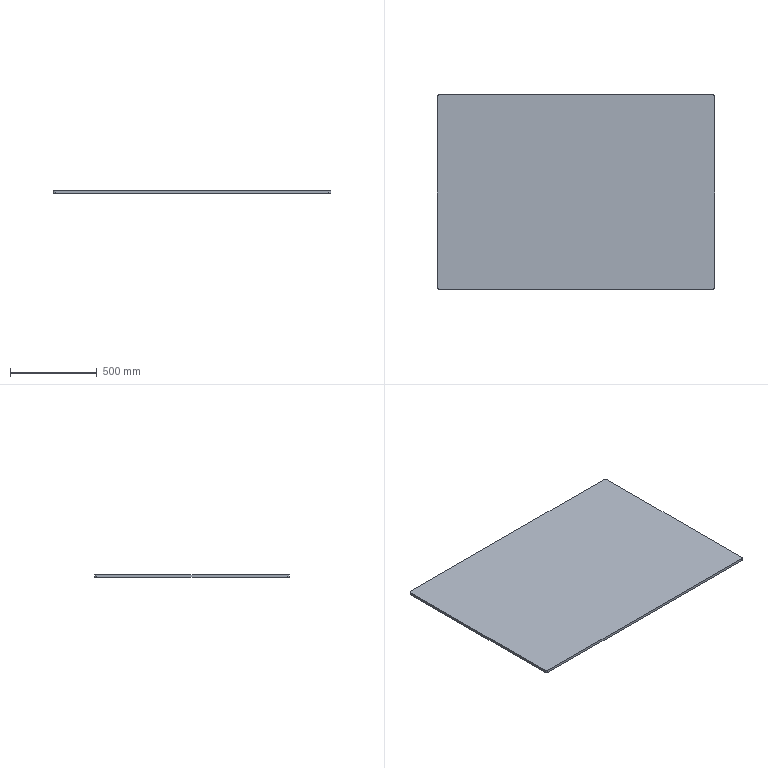Part | STEP file | Part 2 | 1 solid | 10 faces | box 1600 x 1120 x 15 mm | volume 26878712 mm3 | plane 6 | cylinder 4 | commonest cylinder face diameters 20 x4
STEP:
#1=CARTESIAN_POINT('',(800.,-550.,15.));
#2=VERTEX_POINT('',#1);
#3=CARTESIAN_POINT('',(800.,550.,15.));
#4=VERTEX_POINT('',#3);
#5=CARTESIAN_POINT('',(800.,560.,15.));
#6=DIRECTION('',(0.,1.,0.));
#7=VECTOR('',#6,1000.);
#8=LINE('',#5,#7);
#9=EDGE_CURVE('',#2,#4,#8,.T.);
#10=ORIENTED_EDGE('',*,*,#9,.F.);
#11=CARTESIAN_POINT('',(800.,-550.,0.));
#12=VERTEX_POINT('',#11);
#13=CARTESIAN_POINT('',(800.,-550.,15.));
#14=DIRECTION('',(0.,0.,-1.));
#15=VECTOR('',#14,1000.);
#16=LINE('',#13,#15);
#17=EDGE_CURVE('',#2,#12,#16,.T.);
#18=ORIENTED_EDGE('',*,*,#17,.T.);
#19=CARTESIAN_POINT('',(800.,550.,0.));
#20=VERTEX_POINT('',#19);
#21=CARTESIAN_POINT('',(800.,560.,0.));
#22=DIRECTION('',(0.,1.,0.));
#23=VECTOR('',#22,1000.);
#24=LINE('',#21,#23);
#25=EDGE_CURVE('',#12,#20,#24,.T.);
#26=ORIENTED_EDGE('',*,*,#25,.T.);
#27=CARTESIAN_POINT('',(800.,550.,15.));
#28=DIRECTION('',(0.,0.,1.));
#29=VECTOR('',#28,1000.);
#30=LINE('',#27,#29);
#31=EDGE_CURVE('',#20,#4,#30,.T.);
#32=ORIENTED_EDGE('',*,*,#31,.T.);
#33=EDGE_LOOP('',(#10,#18,#26,#32));
#34=FACE_OUTER_BOUND('',#33,.T.);
#35=CARTESIAN_POINT('',(800.,560.,15.));
#36=DIRECTION('',(-1.,0.,0.));
#37=DIRECTION('',(0.,-1.,0.));
#38=AXIS2_PLACEMENT_3D('',#35,#36,#37);
#39=PLANE('',#38);
#40=ADVANCED_FACE('',(#34),#39,.F.);
#41=CARTESIAN_POINT('',(790.,560.,15.));
#42=VERTEX_POINT('',#41);
#43=CARTESIAN_POINT('',(-790.,560.,15.));
#44=VERTEX_POINT('',#43);
#45=CARTESIAN_POINT('',(-800.,560.,15.));
#46=DIRECTION('',(-1.,0.,0.));
#47=VECTOR('',#46,1000.);
#48=LINE('',#45,#47);
#49=EDGE_CURVE('',#42,#44,#48,.T.);
#50=ORIENTED_EDGE('',*,*,#49,.F.);
#51=CARTESIAN_POINT('',(790.,560.,0.));
#52=VERTEX_POINT('',#51);
#53=CARTESIAN_POINT('',(790.,560.,15.));
#54=DIRECTION('',(0.,0.,-1.));
#55=VECTOR('',#54,1000.);
#56=LINE('',#53,#55);
#57=EDGE_CURVE('',#42,#52,#56,.T.);
#58=ORIENTED_EDGE('',*,*,#57,.T.);
#59=CARTESIAN_POINT('',(-790.,560.,0.));
#60=VERTEX_POINT('',#59);
#61=CARTESIAN_POINT('',(-800.,560.,0.));
#62=DIRECTION('',(-1.,0.,0.));
#63=VECTOR('',#62,1000.);
#64=LINE('',#61,#63);
#65=EDGE_CURVE('',#52,#60,#64,.T.);
#66=ORIENTED_EDGE('',*,*,#65,.T.);
#67=CARTESIAN_POINT('',(-790.,560.,15.));
#68=DIRECTION('',(0.,0.,1.));
#69=VECTOR('',#68,1000.);
#70=LINE('',#67,#69);
#71=EDGE_CURVE('',#60,#44,#70,.T.);
#72=ORIENTED_EDGE('',*,*,#71,.T.);
#73=EDGE_LOOP('',(#50,#58,#66,#72));
#74=FACE_OUTER_BOUND('',#73,.T.);
#75=CARTESIAN_POINT('',(-800.,560.,15.));
#76=DIRECTION('',(0.,-1.,0.));
#77=DIRECTION('',(0.,0.,-1.));
#78=AXIS2_PLACEMENT_3D('',#75,#76,#77);
#79=PLANE('',#78);
#80=ADVANCED_FACE('',(#74),#79,.F.);
#81=CARTESIAN_POINT('',(-800.,550.,0.));
#82=VERTEX_POINT('',#81);
#83=CARTESIAN_POINT('',(-800.,-550.,0.));
#84=VERTEX_POINT('',#83);
#85=CARTESIAN_POINT('',(-800.,560.,0.));
#86=DIRECTION('',(0.,-1.,0.));
#87=VECTOR('',#86,1000.);
#88=LINE('',#85,#87);
#89=EDGE_CURVE('',#82,#84,#88,.T.);
#90=ORIENTED_EDGE('',*,*,#89,.T.);
#91=CARTESIAN_POINT('',(-800.,-550.,15.));
#92=VERTEX_POINT('',#91);
#93=CARTESIAN_POINT('',(-800.,-550.,15.));
#94=DIRECTION('',(0.,0.,1.));
#95=VECTOR('',#94,1000.);
#96=LINE('',#93,#95);
#97=EDGE_CURVE('',#84,#92,#96,.T.);
#98=ORIENTED_EDGE('',*,*,#97,.T.);
#99=CARTESIAN_POINT('',(-800.,550.,15.));
#100=VERTEX_POINT('',#99);
#101=CARTESIAN_POINT('',(-800.,560.,15.));
#102=DIRECTION('',(0.,-1.,0.));
#103=VECTOR('',#102,1000.);
#104=LINE('',#101,#103);
#105=EDGE_CURVE('',#100,#92,#104,.T.);
#106=ORIENTED_EDGE('',*,*,#105,.F.);
#107=CARTESIAN_POINT('',(-800.,550.,15.));
#108=DIRECTION('',(0.,0.,-1.));
#109=VECTOR('',#108,1000.);
#110=LINE('',#107,#109);
#111=EDGE_CURVE('',#100,#82,#110,.T.);
#112=ORIENTED_EDGE('',*,*,#111,.T.);
#113=EDGE_LOOP('',(#90,#98,#106,#112));
#114=FACE_OUTER_BOUND('',#113,.T.);
#115=CARTESIAN_POINT('',(-800.,560.,15.));
#116=DIRECTION('',(1.,0.,0.));
#117=DIRECTION('',(0.,0.,-1.));
#118=AXIS2_PLACEMENT_3D('',#115,#116,#117);
#119=PLANE('',#118);
#120=ADVANCED_FACE('',(#114),#119,.F.);
#121=CARTESIAN_POINT('',(-790.,-560.,0.));
#122=VERTEX_POINT('',#121);
#123=CARTESIAN_POINT('',(790.,-560.,0.));
#124=VERTEX_POINT('',#123);
#125=CARTESIAN_POINT('',(-800.,-560.,0.));
#126=DIRECTION('',(1.,0.,0.));
#127=VECTOR('',#126,1000.);
#128=LINE('',#125,#127);
#129=EDGE_CURVE('',#122,#124,#128,.T.);
#130=ORIENTED_EDGE('',*,*,#129,.T.);
#131=CARTESIAN_POINT('',(790.,-560.,15.));
#132=VERTEX_POINT('',#131);
#133=CARTESIAN_POINT('',(790.,-560.,15.));
#134=DIRECTION('',(0.,0.,1.));
#135=VECTOR('',#134,1000.);
#136=LINE('',#133,#135);
#137=EDGE_CURVE('',#124,#132,#136,.T.);
#138=ORIENTED_EDGE('',*,*,#137,.T.);
#139=CARTESIAN_POINT('',(-790.,-560.,15.));
#140=VERTEX_POINT('',#139);
#141=CARTESIAN_POINT('',(-800.,-560.,15.));
#142=DIRECTION('',(1.,0.,0.));
#143=VECTOR('',#142,1000.);
#144=LINE('',#141,#143);
#145=EDGE_CURVE('',#140,#132,#144,.T.);
#146=ORIENTED_EDGE('',*,*,#145,.F.);
#147=CARTESIAN_POINT('',(-790.,-560.,15.));
#148=DIRECTION('',(0.,0.,-1.));
#149=VECTOR('',#148,1000.);
#150=LINE('',#147,#149);
#151=EDGE_CURVE('',#140,#122,#150,.T.);
#152=ORIENTED_EDGE('',*,*,#151,.T.);
#153=EDGE_LOOP('',(#130,#138,#146,#152));
#154=FACE_OUTER_BOUND('',#153,.T.);
#155=CARTESIAN_POINT('',(-800.,-560.,15.));
#156=DIRECTION('',(0.,1.,0.));
#157=DIRECTION('',(0.,0.,1.));
#158=AXIS2_PLACEMENT_3D('',#155,#156,#157);
#159=PLANE('',#158);
#160=ADVANCED_FACE('',(#154),#159,.F.);
#161=ORIENTED_EDGE('',*,*,#145,.T.);
#162=CARTESIAN_POINT('',(790.,-550.,15.));
#163=DIRECTION('',(0.,0.,1.));
#164=DIRECTION('',(1.,0.,0.));
#165=AXIS2_PLACEMENT_3D('',#162,#163,#164);
#166=CIRCLE('',#165,10.);
#167=EDGE_CURVE('',#132,#2,#166,.T.);
#168=ORIENTED_EDGE('',*,*,#167,.T.);
#169=ORIENTED_EDGE('',*,*,#9,.T.);
#170=CARTESIAN_POINT('',(790.,550.,15.));
#171=DIRECTION('',(0.,0.,1.));
#172=DIRECTION('',(1.,0.,0.));
#173=AXIS2_PLACEMENT_3D('',#170,#171,#172);
#174=CIRCLE('',#173,10.);
#175=EDGE_CURVE('',#4,#42,#174,.T.);
#176=ORIENTED_EDGE('',*,*,#175,.T.);
#177=ORIENTED_EDGE('',*,*,#49,.T.);
#178=CARTESIAN_POINT('',(-790.,550.,15.));
#179=DIRECTION('',(0.,0.,1.));
#180=DIRECTION('',(1.,0.,0.));
#181=AXIS2_PLACEMENT_3D('',#178,#179,#180);
#182=CIRCLE('',#181,10.);
#183=EDGE_CURVE('',#44,#100,#182,.T.);
#184=ORIENTED_EDGE('',*,*,#183,.T.);
#185=ORIENTED_EDGE('',*,*,#105,.T.);
#186=CARTESIAN_POINT('',(-790.,-550.,15.));
#187=DIRECTION('',(0.,0.,1.));
#188=DIRECTION('',(1.,0.,0.));
#189=AXIS2_PLACEMENT_3D('',#186,#187,#188);
#190=CIRCLE('',#189,10.);
#191=EDGE_CURVE('',#92,#140,#190,.T.);
#192=ORIENTED_EDGE('',*,*,#191,.T.);
#193=EDGE_LOOP('',(#161,#168,#169,#176,#177,#184,#185,#192));
#194=FACE_OUTER_BOUND('',#193,.T.);
#195=CARTESIAN_POINT('',(0.,0.,15.));
#196=DIRECTION('',(0.,0.,1.));
#197=DIRECTION('',(1.,0.,0.));
#198=AXIS2_PLACEMENT_3D('',#195,#196,#197);
#199=PLANE('',#198);
#200=ADVANCED_FACE('',(#194),#199,.T.);
#201=ORIENTED_EDGE('',*,*,#25,.F.);
#202=CARTESIAN_POINT('',(790.,-550.,0.));
#203=DIRECTION('',(0.,0.,-1.));
#204=DIRECTION('',(1.,0.,0.));
#205=AXIS2_PLACEMENT_3D('',#202,#203,#204);
#206=CIRCLE('',#205,10.);
#207=EDGE_CURVE('',#12,#124,#206,.T.);
#208=ORIENTED_EDGE('',*,*,#207,.T.);
#209=ORIENTED_EDGE('',*,*,#129,.F.);
#210=CARTESIAN_POINT('',(-790.,-550.,0.));
#211=DIRECTION('',(0.,0.,-1.));
#212=DIRECTION('',(1.,0.,0.));
#213=AXIS2_PLACEMENT_3D('',#210,#211,#212);
#214=CIRCLE('',#213,10.);
#215=EDGE_CURVE('',#122,#84,#214,.T.);
#216=ORIENTED_EDGE('',*,*,#215,.T.);
#217=ORIENTED_EDGE('',*,*,#89,.F.);
#218=CARTESIAN_POINT('',(-790.,550.,0.));
#219=DIRECTION('',(0.,0.,-1.));
#220=DIRECTION('',(1.,0.,0.));
#221=AXIS2_PLACEMENT_3D('',#218,#219,#220);
#222=CIRCLE('',#221,10.);
#223=EDGE_CURVE('',#82,#60,#222,.T.);
#224=ORIENTED_EDGE('',*,*,#223,.T.);
#225=ORIENTED_EDGE('',*,*,#65,.F.);
#226=CARTESIAN_POINT('',(790.,550.,0.));
#227=DIRECTION('',(0.,0.,-1.));
#228=DIRECTION('',(1.,0.,0.));
#229=AXIS2_PLACEMENT_3D('',#226,#227,#228);
#230=CIRCLE('',#229,10.);
#231=EDGE_CURVE('',#52,#20,#230,.T.);
#232=ORIENTED_EDGE('',*,*,#231,.T.);
#233=EDGE_LOOP('',(#201,#208,#209,#216,#217,#224,#225,#232));
#234=FACE_OUTER_BOUND('',#233,.T.);
#235=CARTESIAN_POINT('',(0.,0.,0.));
#236=DIRECTION('',(0.,0.,1.));
#237=DIRECTION('',(1.,0.,0.));
#238=AXIS2_PLACEMENT_3D('',#235,#236,#237);
#239=PLANE('',#238);
#240=ADVANCED_FACE('',(#234),#239,.F.);
#241=ORIENTED_EDGE('',*,*,#167,.F.);
#242=ORIENTED_EDGE('',*,*,#137,.F.);
#243=ORIENTED_EDGE('',*,*,#207,.F.);
#244=ORIENTED_EDGE('',*,*,#17,.F.);
#245=EDGE_LOOP('',(#241,#242,#243,#244));
#246=FACE_OUTER_BOUND('',#245,.T.);
#247=CARTESIAN_POINT('',(790.,-550.,15.));
#248=DIRECTION('',(0.,0.,-1.));
#249=DIRECTION('',(-1.,0.,0.));
#250=AXIS2_PLACEMENT_3D('',#247,#248,#249);
#251=CYLINDRICAL_SURFACE('',#250,10.);
#252=ADVANCED_FACE('',(#246),#251,.T.);
#253=ORIENTED_EDGE('',*,*,#175,.F.);
#254=ORIENTED_EDGE('',*,*,#31,.F.);
#255=ORIENTED_EDGE('',*,*,#231,.F.);
#256=ORIENTED_EDGE('',*,*,#57,.F.);
#257=EDGE_LOOP('',(#253,#254,#255,#256));
#258=FACE_OUTER_BOUND('',#257,.T.);
#259=CARTESIAN_POINT('',(790.,550.,15.));
#260=DIRECTION('',(0.,0.,-1.));
#261=DIRECTION('',(-1.,0.,0.));
#262=AXIS2_PLACEMENT_3D('',#259,#260,#261);
#263=CYLINDRICAL_SURFACE('',#262,10.);
#264=ADVANCED_FACE('',(#258),#263,.T.);
#265=ORIENTED_EDGE('',*,*,#191,.F.);
#266=ORIENTED_EDGE('',*,*,#97,.F.);
#267=ORIENTED_EDGE('',*,*,#215,.F.);
#268=ORIENTED_EDGE('',*,*,#151,.F.);
#269=EDGE_LOOP('',(#265,#266,#267,#268));
#270=FACE_OUTER_BOUND('',#269,.T.);
#271=CARTESIAN_POINT('',(-790.,-550.,15.));
#272=DIRECTION('',(0.,0.,-1.));
#273=DIRECTION('',(-1.,0.,0.));
#274=AXIS2_PLACEMENT_3D('',#271,#272,#273);
#275=CYLINDRICAL_SURFACE('',#274,10.);
#276=ADVANCED_FACE('',(#270),#275,.T.);
#277=ORIENTED_EDGE('',*,*,#183,.F.);
#278=ORIENTED_EDGE('',*,*,#71,.F.);
#279=ORIENTED_EDGE('',*,*,#223,.F.);
#280=ORIENTED_EDGE('',*,*,#111,.F.);
#281=EDGE_LOOP('',(#277,#278,#279,#280));
#282=FACE_OUTER_BOUND('',#281,.T.);
#283=CARTESIAN_POINT('',(-790.,550.,15.));
#284=DIRECTION('',(0.,0.,-1.));
#285=DIRECTION('',(-1.,0.,0.));
#286=AXIS2_PLACEMENT_3D('',#283,#284,#285);
#287=CYLINDRICAL_SURFACE('',#286,10.);
#288=ADVANCED_FACE('',(#282),#287,.T.);
#289=CLOSED_SHELL('',(#40,#80,#120,#160,#200,#240,#252,#264,#276,#288));
#290=MANIFOLD_SOLID_BREP('',#289);
#291=CARTESIAN_POINT('',(0.,0.,0.));
#292=DIRECTION('',(0.,0.,1.));
#293=DIRECTION('',(1.,0.,0.));
#294=AXIS2_PLACEMENT_3D('',#291,#292,#293);
#295=(LENGTH_UNIT()NAMED_UNIT(*)SI_UNIT(.MILLI.,.METRE.));
#296=UNCERTAINTY_MEASURE_WITH_UNIT(LENGTH_MEASURE(0.00001),#295,'','');
#297=(NAMED_UNIT(*)PLANE_ANGLE_UNIT()SI_UNIT($,.RADIAN.));
#298=(NAMED_UNIT(*)SI_UNIT($,.STERADIAN.)SOLID_ANGLE_UNIT());
#299=(GEOMETRIC_REPRESENTATION_CONTEXT(3)GLOBAL_UNCERTAINTY_ASSIGNED_CONTEXT((#296))GLOBAL_UNIT_ASSIGNED_CONTEXT((#295,#297,#298))REPRESENTATION_CONTEXT('',''));
#300=ADVANCED_BREP_SHAPE_REPRESENTATION('',(#290,#294),#299);